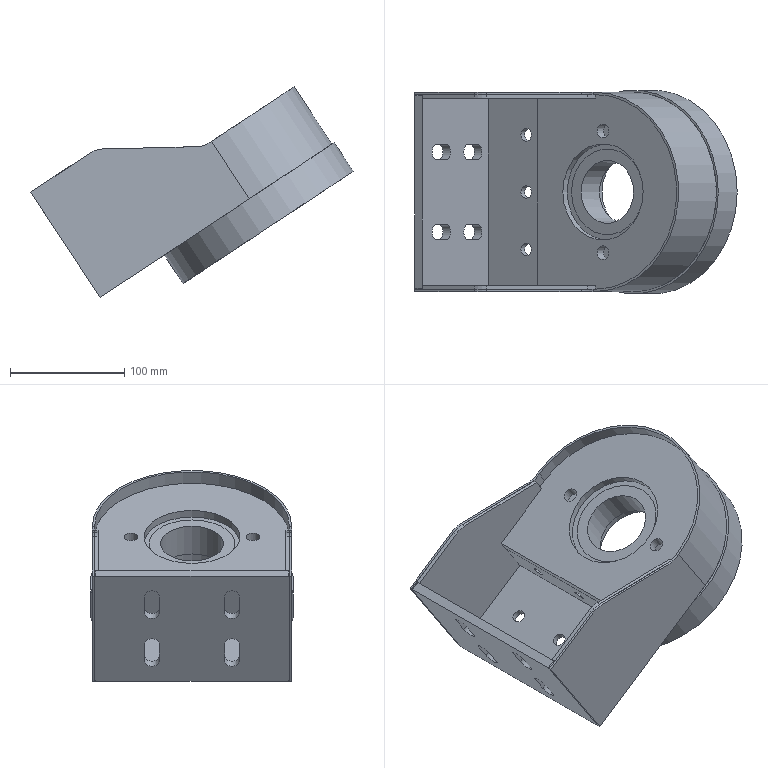Part | STEP file | HL4GZ-1.862.035 (motor mounting bracket weldment) | 9 solids | 114 faces | box 281.601 x 178 x 183.899 mm | volume 825391 mm3 | plane 70 | cylinder 42 | cone 2 | commonest cylinder face diameters 13 x8 40 x6 11 x5 2 x4 9 x3 170 x3